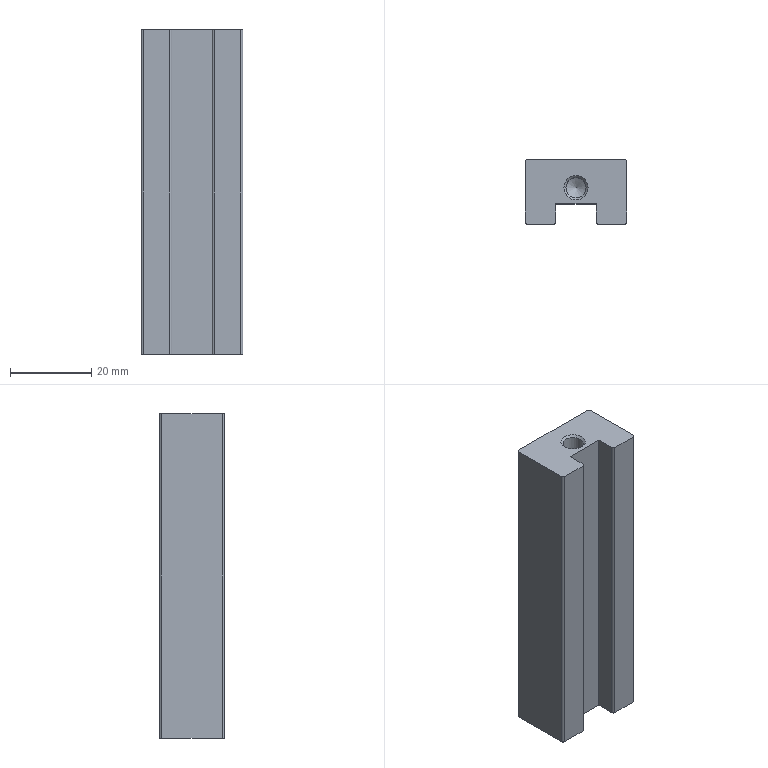Part | STEP file | 200 mesh_id1982 | 1 solid | 19 faces | box 25 x 16 x 80 mm | volume 27373 mm3 | plane 10 | cylinder 7 | cone 2 | commonest cylinder face diameters 1 x6 5 x1
STEP:
#1=CARTESIAN_POINT('',(-17200.384,-3959.169,0.));
#2=VERTEX_POINT('',#1);
#3=CARTESIAN_POINT('',(-17200.384,-3974.169,0.));
#4=VERTEX_POINT('',#3);
#5=CARTESIAN_POINT('',(-17200.384,-3959.169,0.));
#6=DIRECTION('',(0.,-1.,0.));
#7=VECTOR('',#6,1.);
#8=LINE('',#5,#7);
#9=EDGE_CURVE('',#2,#4,#8,.T.);
#10=ORIENTED_EDGE('',*,*,#9,.F.);
#11=CARTESIAN_POINT('',(-17200.384,-3959.169,80.));
#12=VERTEX_POINT('',#11);
#13=CARTESIAN_POINT('',(-17200.384,-3959.169,80.));
#14=DIRECTION('',(0.,0.,-1.));
#15=VECTOR('',#14,1.);
#16=LINE('',#13,#15);
#17=EDGE_CURVE('',#12,#2,#16,.T.);
#18=ORIENTED_EDGE('',*,*,#17,.F.);
#19=CARTESIAN_POINT('',(-17200.384,-3974.169,80.));
#20=VERTEX_POINT('',#19);
#21=CARTESIAN_POINT('',(-17200.384,-3959.169,80.));
#22=DIRECTION('',(0.,-1.,0.));
#23=VECTOR('',#22,1.);
#24=LINE('',#21,#23);
#25=EDGE_CURVE('',#12,#20,#24,.T.);
#26=ORIENTED_EDGE('',*,*,#25,.T.);
#27=CARTESIAN_POINT('',(-17200.384,-3974.169,80.));
#28=DIRECTION('',(0.,0.,-1.));
#29=VECTOR('',#28,1.);
#30=LINE('',#27,#29);
#31=EDGE_CURVE('',#20,#4,#30,.T.);
#32=ORIENTED_EDGE('',*,*,#31,.T.);
#33=EDGE_LOOP('',(#10,#18,#26,#32));
#34=FACE_OUTER_BOUND('',#33,.T.);
#35=CARTESIAN_POINT('',(-17200.384,-3959.169,80.));
#36=DIRECTION('',(1.,0.,0.));
#37=DIRECTION('',(0.,0.,1.));
#38=AXIS2_PLACEMENT_3D('',#35,#36,#37);
#39=PLANE('',#38);
#40=ADVANCED_FACE('',(#34),#39,.T.);
#41=CARTESIAN_POINT('',(-17200.884,-3974.669,0.));
#42=VERTEX_POINT('',#41);
#43=CARTESIAN_POINT('',(-17200.884,-3974.169,0.));
#44=DIRECTION('',(0.,0.,-1.));
#45=DIRECTION('',(1.,0.,0.));
#46=AXIS2_PLACEMENT_3D('',#43,#44,#45);
#47=CIRCLE('',#46,0.5);
#48=EDGE_CURVE('',#4,#42,#47,.T.);
#49=ORIENTED_EDGE('',*,*,#48,.F.);
#50=ORIENTED_EDGE('',*,*,#31,.F.);
#51=CARTESIAN_POINT('',(-17200.884,-3974.669,80.));
#52=VERTEX_POINT('',#51);
#53=CARTESIAN_POINT('',(-17200.884,-3974.169,80.));
#54=DIRECTION('',(0.,0.,-1.));
#55=DIRECTION('',(1.,0.,0.));
#56=AXIS2_PLACEMENT_3D('',#53,#54,#55);
#57=CIRCLE('',#56,0.5);
#58=EDGE_CURVE('',#20,#52,#57,.T.);
#59=ORIENTED_EDGE('',*,*,#58,.T.);
#60=CARTESIAN_POINT('',(-17200.884,-3974.669,80.));
#61=DIRECTION('',(0.,0.,-1.));
#62=VECTOR('',#61,1.);
#63=LINE('',#60,#62);
#64=EDGE_CURVE('',#52,#42,#63,.T.);
#65=ORIENTED_EDGE('',*,*,#64,.T.);
#66=EDGE_LOOP('',(#49,#50,#59,#65));
#67=FACE_OUTER_BOUND('',#66,.T.);
#68=CARTESIAN_POINT('',(-17200.884,-3974.169,80.));
#69=DIRECTION('',(0.,0.,-1.));
#70=DIRECTION('',(1.,0.,0.));
#71=AXIS2_PLACEMENT_3D('',#68,#69,#70);
#72=CYLINDRICAL_SURFACE('',#71,0.5);
#73=ADVANCED_FACE('',(#67),#72,.T.);
#74=CARTESIAN_POINT('',(-17207.384,-3974.669,0.));
#75=VERTEX_POINT('',#74);
#76=CARTESIAN_POINT('',(-17200.884,-3974.669,0.));
#77=DIRECTION('',(-1.,0.,0.));
#78=VECTOR('',#77,1.);
#79=LINE('',#76,#78);
#80=EDGE_CURVE('',#42,#75,#79,.T.);
#81=ORIENTED_EDGE('',*,*,#80,.F.);
#82=ORIENTED_EDGE('',*,*,#64,.F.);
#83=CARTESIAN_POINT('',(-17207.384,-3974.669,80.));
#84=VERTEX_POINT('',#83);
#85=CARTESIAN_POINT('',(-17200.884,-3974.669,80.));
#86=DIRECTION('',(-1.,0.,0.));
#87=VECTOR('',#86,1.);
#88=LINE('',#85,#87);
#89=EDGE_CURVE('',#52,#84,#88,.T.);
#90=ORIENTED_EDGE('',*,*,#89,.T.);
#91=CARTESIAN_POINT('',(-17207.384,-3974.669,80.));
#92=DIRECTION('',(0.,0.,-1.));
#93=VECTOR('',#92,1.);
#94=LINE('',#91,#93);
#95=EDGE_CURVE('',#84,#75,#94,.T.);
#96=ORIENTED_EDGE('',*,*,#95,.T.);
#97=EDGE_LOOP('',(#81,#82,#90,#96));
#98=FACE_OUTER_BOUND('',#97,.T.);
#99=CARTESIAN_POINT('',(-17200.884,-3974.669,80.));
#100=DIRECTION('',(0.,-1.,0.));
#101=DIRECTION('',(0.,0.,1.));
#102=AXIS2_PLACEMENT_3D('',#99,#100,#101);
#103=PLANE('',#102);
#104=ADVANCED_FACE('',(#98),#103,.T.);
#105=CARTESIAN_POINT('',(-17207.884,-3974.169,0.));
#106=VERTEX_POINT('',#105);
#107=CARTESIAN_POINT('',(-17207.384,-3974.169,0.));
#108=DIRECTION('',(0.,0.,-1.));
#109=DIRECTION('',(1.,0.,0.));
#110=AXIS2_PLACEMENT_3D('',#107,#108,#109);
#111=CIRCLE('',#110,0.5);
#112=EDGE_CURVE('',#75,#106,#111,.T.);
#113=ORIENTED_EDGE('',*,*,#112,.F.);
#114=ORIENTED_EDGE('',*,*,#95,.F.);
#115=CARTESIAN_POINT('',(-17207.884,-3974.169,80.));
#116=VERTEX_POINT('',#115);
#117=CARTESIAN_POINT('',(-17207.384,-3974.169,80.));
#118=DIRECTION('',(0.,0.,-1.));
#119=DIRECTION('',(1.,0.,0.));
#120=AXIS2_PLACEMENT_3D('',#117,#118,#119);
#121=CIRCLE('',#120,0.5);
#122=EDGE_CURVE('',#84,#116,#121,.T.);
#123=ORIENTED_EDGE('',*,*,#122,.T.);
#124=CARTESIAN_POINT('',(-17207.884,-3974.169,80.));
#125=DIRECTION('',(0.,0.,-1.));
#126=VECTOR('',#125,1.);
#127=LINE('',#124,#126);
#128=EDGE_CURVE('',#116,#106,#127,.T.);
#129=ORIENTED_EDGE('',*,*,#128,.T.);
#130=EDGE_LOOP('',(#113,#114,#123,#129));
#131=FACE_OUTER_BOUND('',#130,.T.);
#132=CARTESIAN_POINT('',(-17207.384,-3974.169,80.));
#133=DIRECTION('',(0.,0.,-1.));
#134=DIRECTION('',(1.,0.,0.));
#135=AXIS2_PLACEMENT_3D('',#132,#133,#134);
#136=CYLINDRICAL_SURFACE('',#135,0.5);
#137=ADVANCED_FACE('',(#131),#136,.T.);
#138=CARTESIAN_POINT('',(-17207.884,-3969.669,0.));
#139=VERTEX_POINT('',#138);
#140=CARTESIAN_POINT('',(-17207.884,-3974.169,0.));
#141=DIRECTION('',(0.,1.,0.));
#142=VECTOR('',#141,1.);
#143=LINE('',#140,#142);
#144=EDGE_CURVE('',#106,#139,#143,.T.);
#145=ORIENTED_EDGE('',*,*,#144,.F.);
#146=ORIENTED_EDGE('',*,*,#128,.F.);
#147=CARTESIAN_POINT('',(-17207.884,-3969.669,80.));
#148=VERTEX_POINT('',#147);
#149=CARTESIAN_POINT('',(-17207.884,-3974.169,80.));
#150=DIRECTION('',(0.,1.,0.));
#151=VECTOR('',#150,1.);
#152=LINE('',#149,#151);
#153=EDGE_CURVE('',#116,#148,#152,.T.);
#154=ORIENTED_EDGE('',*,*,#153,.T.);
#155=CARTESIAN_POINT('',(-17207.884,-3969.669,80.));
#156=DIRECTION('',(0.,0.,-1.));
#157=VECTOR('',#156,1.);
#158=LINE('',#155,#157);
#159=EDGE_CURVE('',#148,#139,#158,.T.);
#160=ORIENTED_EDGE('',*,*,#159,.T.);
#161=EDGE_LOOP('',(#145,#146,#154,#160));
#162=FACE_OUTER_BOUND('',#161,.T.);
#163=CARTESIAN_POINT('',(-17207.884,-3974.169,80.));
#164=DIRECTION('',(-1.,0.,0.));
#165=DIRECTION('',(0.,0.,-1.));
#166=AXIS2_PLACEMENT_3D('',#163,#164,#165);
#167=PLANE('',#166);
#168=ADVANCED_FACE('',(#162),#167,.T.);
#169=CARTESIAN_POINT('',(-17217.884,-3969.669,0.));
#170=VERTEX_POINT('',#169);
#171=CARTESIAN_POINT('',(-17207.884,-3969.669,0.));
#172=DIRECTION('',(-1.,0.,0.));
#173=VECTOR('',#172,1.);
#174=LINE('',#171,#173);
#175=EDGE_CURVE('',#139,#170,#174,.T.);
#176=ORIENTED_EDGE('',*,*,#175,.F.);
#177=ORIENTED_EDGE('',*,*,#159,.F.);
#178=CARTESIAN_POINT('',(-17217.884,-3969.669,80.));
#179=VERTEX_POINT('',#178);
#180=CARTESIAN_POINT('',(-17207.884,-3969.669,80.));
#181=DIRECTION('',(-1.,0.,0.));
#182=VECTOR('',#181,1.);
#183=LINE('',#180,#182);
#184=EDGE_CURVE('',#148,#179,#183,.T.);
#185=ORIENTED_EDGE('',*,*,#184,.T.);
#186=CARTESIAN_POINT('',(-17217.884,-3969.669,80.));
#187=DIRECTION('',(0.,0.,-1.));
#188=VECTOR('',#187,1.);
#189=LINE('',#186,#188);
#190=EDGE_CURVE('',#179,#170,#189,.T.);
#191=ORIENTED_EDGE('',*,*,#190,.T.);
#192=EDGE_LOOP('',(#176,#177,#185,#191));
#193=FACE_OUTER_BOUND('',#192,.T.);
#194=CARTESIAN_POINT('',(-17207.884,-3969.669,80.));
#195=DIRECTION('',(0.,-1.,0.));
#196=DIRECTION('',(0.,0.,1.));
#197=AXIS2_PLACEMENT_3D('',#194,#195,#196);
#198=PLANE('',#197);
#199=ADVANCED_FACE('',(#193),#198,.T.);
#200=CARTESIAN_POINT('',(-17217.884,-3974.169,0.));
#201=VERTEX_POINT('',#200);
#202=CARTESIAN_POINT('',(-17217.884,-3969.669,0.));
#203=DIRECTION('',(0.,-1.,0.));
#204=VECTOR('',#203,1.);
#205=LINE('',#202,#204);
#206=EDGE_CURVE('',#170,#201,#205,.T.);
#207=ORIENTED_EDGE('',*,*,#206,.F.);
#208=ORIENTED_EDGE('',*,*,#190,.F.);
#209=CARTESIAN_POINT('',(-17217.884,-3974.169,80.));
#210=VERTEX_POINT('',#209);
#211=CARTESIAN_POINT('',(-17217.884,-3969.669,80.));
#212=DIRECTION('',(0.,-1.,0.));
#213=VECTOR('',#212,1.);
#214=LINE('',#211,#213);
#215=EDGE_CURVE('',#179,#210,#214,.T.);
#216=ORIENTED_EDGE('',*,*,#215,.T.);
#217=CARTESIAN_POINT('',(-17217.884,-3974.169,80.));
#218=DIRECTION('',(0.,0.,-1.));
#219=VECTOR('',#218,1.);
#220=LINE('',#217,#219);
#221=EDGE_CURVE('',#210,#201,#220,.T.);
#222=ORIENTED_EDGE('',*,*,#221,.T.);
#223=EDGE_LOOP('',(#207,#208,#216,#222));
#224=FACE_OUTER_BOUND('',#223,.T.);
#225=CARTESIAN_POINT('',(-17217.884,-3969.669,80.));
#226=DIRECTION('',(1.,0.,0.));
#227=DIRECTION('',(0.,0.,1.));
#228=AXIS2_PLACEMENT_3D('',#225,#226,#227);
#229=PLANE('',#228);
#230=ADVANCED_FACE('',(#224),#229,.T.);
#231=CARTESIAN_POINT('',(-17218.384,-3974.669,0.));
#232=VERTEX_POINT('',#231);
#233=CARTESIAN_POINT('',(-17218.384,-3974.169,0.));
#234=DIRECTION('',(0.,0.,-1.));
#235=DIRECTION('',(1.,0.,0.));
#236=AXIS2_PLACEMENT_3D('',#233,#234,#235);
#237=CIRCLE('',#236,0.5);
#238=EDGE_CURVE('',#201,#232,#237,.T.);
#239=ORIENTED_EDGE('',*,*,#238,.F.);
#240=ORIENTED_EDGE('',*,*,#221,.F.);
#241=CARTESIAN_POINT('',(-17218.384,-3974.669,80.));
#242=VERTEX_POINT('',#241);
#243=CARTESIAN_POINT('',(-17218.384,-3974.169,80.));
#244=DIRECTION('',(0.,0.,-1.));
#245=DIRECTION('',(1.,0.,0.));
#246=AXIS2_PLACEMENT_3D('',#243,#244,#245);
#247=CIRCLE('',#246,0.5);
#248=EDGE_CURVE('',#210,#242,#247,.T.);
#249=ORIENTED_EDGE('',*,*,#248,.T.);
#250=CARTESIAN_POINT('',(-17218.384,-3974.669,80.));
#251=DIRECTION('',(0.,0.,-1.));
#252=VECTOR('',#251,1.);
#253=LINE('',#250,#252);
#254=EDGE_CURVE('',#242,#232,#253,.T.);
#255=ORIENTED_EDGE('',*,*,#254,.T.);
#256=EDGE_LOOP('',(#239,#240,#249,#255));
#257=FACE_OUTER_BOUND('',#256,.T.);
#258=CARTESIAN_POINT('',(-17218.384,-3974.169,80.));
#259=DIRECTION('',(0.,0.,-1.));
#260=DIRECTION('',(1.,0.,0.));
#261=AXIS2_PLACEMENT_3D('',#258,#259,#260);
#262=CYLINDRICAL_SURFACE('',#261,0.5);
#263=ADVANCED_FACE('',(#257),#262,.T.);
#264=CARTESIAN_POINT('',(-17224.884,-3974.669,0.));
#265=VERTEX_POINT('',#264);
#266=CARTESIAN_POINT('',(-17218.384,-3974.669,0.));
#267=DIRECTION('',(-1.,0.,0.));
#268=VECTOR('',#267,1.);
#269=LINE('',#266,#268);
#270=EDGE_CURVE('',#232,#265,#269,.T.);
#271=ORIENTED_EDGE('',*,*,#270,.F.);
#272=ORIENTED_EDGE('',*,*,#254,.F.);
#273=CARTESIAN_POINT('',(-17224.884,-3974.669,80.));
#274=VERTEX_POINT('',#273);
#275=CARTESIAN_POINT('',(-17218.384,-3974.669,80.));
#276=DIRECTION('',(-1.,0.,0.));
#277=VECTOR('',#276,1.);
#278=LINE('',#275,#277);
#279=EDGE_CURVE('',#242,#274,#278,.T.);
#280=ORIENTED_EDGE('',*,*,#279,.T.);
#281=CARTESIAN_POINT('',(-17224.884,-3974.669,80.));
#282=DIRECTION('',(0.,0.,-1.));
#283=VECTOR('',#282,1.);
#284=LINE('',#281,#283);
#285=EDGE_CURVE('',#274,#265,#284,.T.);
#286=ORIENTED_EDGE('',*,*,#285,.T.);
#287=EDGE_LOOP('',(#271,#272,#280,#286));
#288=FACE_OUTER_BOUND('',#287,.T.);
#289=CARTESIAN_POINT('',(-17218.384,-3974.669,80.));
#290=DIRECTION('',(0.,-1.,0.));
#291=DIRECTION('',(0.,0.,1.));
#292=AXIS2_PLACEMENT_3D('',#289,#290,#291);
#293=PLANE('',#292);
#294=ADVANCED_FACE('',(#288),#293,.T.);
#295=CARTESIAN_POINT('',(-17225.384,-3974.169,0.));
#296=VERTEX_POINT('',#295);
#297=CARTESIAN_POINT('',(-17224.884,-3974.169,0.));
#298=DIRECTION('',(0.,0.,-1.));
#299=DIRECTION('',(1.,0.,0.));
#300=AXIS2_PLACEMENT_3D('',#297,#298,#299);
#301=CIRCLE('',#300,0.5);
#302=EDGE_CURVE('',#265,#296,#301,.T.);
#303=ORIENTED_EDGE('',*,*,#302,.F.);
#304=ORIENTED_EDGE('',*,*,#285,.F.);
#305=CARTESIAN_POINT('',(-17225.384,-3974.169,80.));
#306=VERTEX_POINT('',#305);
#307=CARTESIAN_POINT('',(-17224.884,-3974.169,80.));
#308=DIRECTION('',(0.,0.,-1.));
#309=DIRECTION('',(1.,0.,0.));
#310=AXIS2_PLACEMENT_3D('',#307,#308,#309);
#311=CIRCLE('',#310,0.5);
#312=EDGE_CURVE('',#274,#306,#311,.T.);
#313=ORIENTED_EDGE('',*,*,#312,.T.);
#314=CARTESIAN_POINT('',(-17225.384,-3974.169,80.));
#315=DIRECTION('',(0.,0.,-1.));
#316=VECTOR('',#315,1.);
#317=LINE('',#314,#316);
#318=EDGE_CURVE('',#306,#296,#317,.T.);
#319=ORIENTED_EDGE('',*,*,#318,.T.);
#320=EDGE_LOOP('',(#303,#304,#313,#319));
#321=FACE_OUTER_BOUND('',#320,.T.);
#322=CARTESIAN_POINT('',(-17224.884,-3974.169,80.));
#323=DIRECTION('',(0.,0.,-1.));
#324=DIRECTION('',(1.,0.,0.));
#325=AXIS2_PLACEMENT_3D('',#322,#323,#324);
#326=CYLINDRICAL_SURFACE('',#325,0.5);
#327=ADVANCED_FACE('',(#321),#326,.T.);
#328=CARTESIAN_POINT('',(-17225.384,-3959.169,0.));
#329=VERTEX_POINT('',#328);
#330=CARTESIAN_POINT('',(-17225.384,-3974.169,0.));
#331=DIRECTION('',(0.,1.,0.));
#332=VECTOR('',#331,1.);
#333=LINE('',#330,#332);
#334=EDGE_CURVE('',#296,#329,#333,.T.);
#335=ORIENTED_EDGE('',*,*,#334,.F.);
#336=ORIENTED_EDGE('',*,*,#318,.F.);
#337=CARTESIAN_POINT('',(-17225.384,-3959.169,80.));
#338=VERTEX_POINT('',#337);
#339=CARTESIAN_POINT('',(-17225.384,-3974.169,80.));
#340=DIRECTION('',(0.,1.,0.));
#341=VECTOR('',#340,1.);
#342=LINE('',#339,#341);
#343=EDGE_CURVE('',#306,#338,#342,.T.);
#344=ORIENTED_EDGE('',*,*,#343,.T.);
#345=CARTESIAN_POINT('',(-17225.384,-3959.169,80.));
#346=DIRECTION('',(0.,0.,-1.));
#347=VECTOR('',#346,1.);
#348=LINE('',#345,#347);
#349=EDGE_CURVE('',#338,#329,#348,.T.);
#350=ORIENTED_EDGE('',*,*,#349,.T.);
#351=EDGE_LOOP('',(#335,#336,#344,#350));
#352=FACE_OUTER_BOUND('',#351,.T.);
#353=CARTESIAN_POINT('',(-17225.384,-3974.169,80.));
#354=DIRECTION('',(-1.,0.,0.));
#355=DIRECTION('',(0.,0.,-1.));
#356=AXIS2_PLACEMENT_3D('',#353,#354,#355);
#357=PLANE('',#356);
#358=ADVANCED_FACE('',(#352),#357,.T.);
#359=CARTESIAN_POINT('',(-17224.884,-3958.669,0.));
#360=VERTEX_POINT('',#359);
#361=CARTESIAN_POINT('',(-17224.884,-3959.169,0.));
#362=DIRECTION('',(0.,0.,-1.));
#363=DIRECTION('',(1.,0.,0.));
#364=AXIS2_PLACEMENT_3D('',#361,#362,#363);
#365=CIRCLE('',#364,0.5);
#366=EDGE_CURVE('',#329,#360,#365,.T.);
#367=ORIENTED_EDGE('',*,*,#366,.F.);
#368=ORIENTED_EDGE('',*,*,#349,.F.);
#369=CARTESIAN_POINT('',(-17224.884,-3958.669,80.));
#370=VERTEX_POINT('',#369);
#371=CARTESIAN_POINT('',(-17224.884,-3959.169,80.));
#372=DIRECTION('',(0.,0.,-1.));
#373=DIRECTION('',(1.,0.,0.));
#374=AXIS2_PLACEMENT_3D('',#371,#372,#373);
#375=CIRCLE('',#374,0.5);
#376=EDGE_CURVE('',#338,#370,#375,.T.);
#377=ORIENTED_EDGE('',*,*,#376,.T.);
#378=CARTESIAN_POINT('',(-17224.884,-3958.669,80.));
#379=DIRECTION('',(0.,0.,-1.));
#380=VECTOR('',#379,1.);
#381=LINE('',#378,#380);
#382=EDGE_CURVE('',#370,#360,#381,.T.);
#383=ORIENTED_EDGE('',*,*,#382,.T.);
#384=EDGE_LOOP('',(#367,#368,#377,#383));
#385=FACE_OUTER_BOUND('',#384,.T.);
#386=CARTESIAN_POINT('',(-17224.884,-3959.169,80.));
#387=DIRECTION('',(0.,0.,-1.));
#388=DIRECTION('',(1.,0.,0.));
#389=AXIS2_PLACEMENT_3D('',#386,#387,#388);
#390=CYLINDRICAL_SURFACE('',#389,0.5);
#391=ADVANCED_FACE('',(#385),#390,.T.);
#392=CARTESIAN_POINT('',(-17200.884,-3958.669,0.));
#393=VERTEX_POINT('',#392);
#394=CARTESIAN_POINT('',(-17224.884,-3958.669,0.));
#395=DIRECTION('',(1.,0.,0.));
#396=VECTOR('',#395,1.);
#397=LINE('',#394,#396);
#398=EDGE_CURVE('',#360,#393,#397,.T.);
#399=ORIENTED_EDGE('',*,*,#398,.F.);
#400=ORIENTED_EDGE('',*,*,#382,.F.);
#401=CARTESIAN_POINT('',(-17200.884,-3958.669,80.));
#402=VERTEX_POINT('',#401);
#403=CARTESIAN_POINT('',(-17224.884,-3958.669,80.));
#404=DIRECTION('',(1.,0.,0.));
#405=VECTOR('',#404,1.);
#406=LINE('',#403,#405);
#407=EDGE_CURVE('',#370,#402,#406,.T.);
#408=ORIENTED_EDGE('',*,*,#407,.T.);
#409=CARTESIAN_POINT('',(-17200.884,-3958.669,80.));
#410=DIRECTION('',(0.,0.,-1.));
#411=VECTOR('',#410,1.);
#412=LINE('',#409,#411);
#413=EDGE_CURVE('',#402,#393,#412,.T.);
#414=ORIENTED_EDGE('',*,*,#413,.T.);
#415=EDGE_LOOP('',(#399,#400,#408,#414));
#416=FACE_OUTER_BOUND('',#415,.T.);
#417=CARTESIAN_POINT('',(-17224.884,-3958.669,80.));
#418=DIRECTION('',(0.,1.,0.));
#419=DIRECTION('',(0.,0.,-1.));
#420=AXIS2_PLACEMENT_3D('',#417,#418,#419);
#421=PLANE('',#420);
#422=ADVANCED_FACE('',(#416),#421,.T.);
#423=CARTESIAN_POINT('',(-17200.884,-3959.169,0.));
#424=DIRECTION('',(0.,0.,-1.));
#425=DIRECTION('',(1.,0.,0.));
#426=AXIS2_PLACEMENT_3D('',#423,#424,#425);
#427=CIRCLE('',#426,0.5);
#428=EDGE_CURVE('',#393,#2,#427,.T.);
#429=ORIENTED_EDGE('',*,*,#428,.F.);
#430=ORIENTED_EDGE('',*,*,#413,.F.);
#431=CARTESIAN_POINT('',(-17200.884,-3959.169,80.));
#432=DIRECTION('',(0.,0.,-1.));
#433=DIRECTION('',(1.,0.,0.));
#434=AXIS2_PLACEMENT_3D('',#431,#432,#433);
#435=CIRCLE('',#434,0.5);
#436=EDGE_CURVE('',#402,#12,#435,.T.);
#437=ORIENTED_EDGE('',*,*,#436,.T.);
#438=ORIENTED_EDGE('',*,*,#17,.T.);
#439=EDGE_LOOP('',(#429,#430,#437,#438));
#440=FACE_OUTER_BOUND('',#439,.T.);
#441=CARTESIAN_POINT('',(-17200.884,-3959.169,80.));
#442=DIRECTION('',(0.,0.,-1.));
#443=DIRECTION('',(1.,0.,0.));
#444=AXIS2_PLACEMENT_3D('',#441,#442,#443);
#445=CYLINDRICAL_SURFACE('',#444,0.5);
#446=ADVANCED_FACE('',(#440),#445,.T.);
#447=CARTESIAN_POINT('',(-17215.884,-3965.669,80.));
#448=VERTEX_POINT('',#447);
#449=CARTESIAN_POINT('',(-17212.884,-3965.669,80.));
#450=DIRECTION('',(0.,0.,-1.));
#451=DIRECTION('',(-1.,0.,0.));
#452=AXIS2_PLACEMENT_3D('',#449,#450,#451);
#453=CIRCLE('',#452,3.);
#454=EDGE_CURVE('',#448,#448,#453,.T.);
#455=ORIENTED_EDGE('',*,*,#454,.T.);
#456=EDGE_LOOP('',(#455));
#457=FACE_BOUND('',#456,.T.);
#458=ORIENTED_EDGE('',*,*,#25,.F.);
#459=ORIENTED_EDGE('',*,*,#436,.F.);
#460=ORIENTED_EDGE('',*,*,#407,.F.);
#461=ORIENTED_EDGE('',*,*,#376,.F.);
#462=ORIENTED_EDGE('',*,*,#343,.F.);
#463=ORIENTED_EDGE('',*,*,#312,.F.);
#464=ORIENTED_EDGE('',*,*,#279,.F.);
#465=ORIENTED_EDGE('',*,*,#248,.F.);
#466=ORIENTED_EDGE('',*,*,#215,.F.);
#467=ORIENTED_EDGE('',*,*,#184,.F.);
#468=ORIENTED_EDGE('',*,*,#153,.F.);
#469=ORIENTED_EDGE('',*,*,#122,.F.);
#470=ORIENTED_EDGE('',*,*,#89,.F.);
#471=ORIENTED_EDGE('',*,*,#58,.F.);
#472=EDGE_LOOP('',(#458,#459,#460,#461,#462,#463,#464,#465,#466,#467,#468,#469,#470,#471));
#473=FACE_BOUND('',#472,.T.);
#474=CARTESIAN_POINT('',(-17200.884,-3974.169,80.));
#475=DIRECTION('',(0.,0.,-1.));
#476=DIRECTION('',(1.,0.,0.));
#477=AXIS2_PLACEMENT_3D('',#474,#475,#476);
#478=PLANE('',#477);
#479=ADVANCED_FACE('',(#457,#473),#478,.F.);
#480=ORIENTED_EDGE('',*,*,#9,.T.);
#481=ORIENTED_EDGE('',*,*,#48,.T.);
#482=ORIENTED_EDGE('',*,*,#80,.T.);
#483=ORIENTED_EDGE('',*,*,#112,.T.);
#484=ORIENTED_EDGE('',*,*,#144,.T.);
#485=ORIENTED_EDGE('',*,*,#175,.T.);
#486=ORIENTED_EDGE('',*,*,#206,.T.);
#487=ORIENTED_EDGE('',*,*,#238,.T.);
#488=ORIENTED_EDGE('',*,*,#270,.T.);
#489=ORIENTED_EDGE('',*,*,#302,.T.);
#490=ORIENTED_EDGE('',*,*,#334,.T.);
#491=ORIENTED_EDGE('',*,*,#366,.T.);
#492=ORIENTED_EDGE('',*,*,#398,.T.);
#493=ORIENTED_EDGE('',*,*,#428,.T.);
#494=EDGE_LOOP('',(#480,#481,#482,#483,#484,#485,#486,#487,#488,#489,#490,#491,#492,#493));
#495=FACE_OUTER_BOUND('',#494,.T.);
#496=CARTESIAN_POINT('',(-17200.884,-3974.169,0.));
#497=DIRECTION('',(0.,0.,-1.));
#498=DIRECTION('',(1.,0.,0.));
#499=AXIS2_PLACEMENT_3D('',#496,#497,#498);
#500=PLANE('',#499);
#501=ADVANCED_FACE('',(#495),#500,.T.);
#502=CARTESIAN_POINT('',(-17215.384,-3965.669,50.));
#503=VERTEX_POINT('',#502);
#504=CARTESIAN_POINT('',(-17212.884,-3965.669,50.));
#505=DIRECTION('',(0.,0.,1.));
#506=DIRECTION('',(-1.,0.,0.));
#507=AXIS2_PLACEMENT_3D('',#504,#505,#506);
#508=CIRCLE('',#507,2.5);
#509=EDGE_CURVE('',#503,#503,#508,.T.);
#510=ORIENTED_EDGE('',*,*,#509,.T.);
#511=EDGE_LOOP('',(#510));
#512=FACE_BOUND('',#511,.T.);
#513=CARTESIAN_POINT('',(-17212.884,-3965.669,48.498));
#514=VERTEX_POINT('',#513);
#515=VERTEX_LOOP('',#514);
#516=FACE_BOUND('',#515,.T.);
#517=CARTESIAN_POINT('',(-17212.884,-3965.669,50.));
#518=DIRECTION('',(0.,0.,1.));
#519=DIRECTION('',(-1.,0.,0.));
#520=AXIS2_PLACEMENT_3D('',#517,#518,#519);
#521=CONICAL_SURFACE('',#520,2.5,59.);
#522=ADVANCED_FACE('',(#512,#516),#521,.F.);
#523=CARTESIAN_POINT('',(-17215.384,-3965.669,79.5));
#524=VERTEX_POINT('',#523);
#525=CARTESIAN_POINT('',(-17212.884,-3965.669,79.5));
#526=DIRECTION('',(0.,0.,1.));
#527=DIRECTION('',(-1.,0.,0.));
#528=AXIS2_PLACEMENT_3D('',#525,#526,#527);
#529=CIRCLE('',#528,2.5);
#530=EDGE_CURVE('',#524,#524,#529,.T.);
#531=ORIENTED_EDGE('',*,*,#530,.T.);
#532=EDGE_LOOP('',(#531));
#533=FACE_BOUND('',#532,.T.);
#534=ORIENTED_EDGE('',*,*,#509,.F.);
#535=EDGE_LOOP('',(#534));
#536=FACE_BOUND('',#535,.T.);
#537=CARTESIAN_POINT('',(-17212.884,-3965.669,80.));
#538=DIRECTION('',(0.,0.,-1.));
#539=DIRECTION('',(1.,0.,0.));
#540=AXIS2_PLACEMENT_3D('',#537,#538,#539);
#541=CYLINDRICAL_SURFACE('',#540,2.5);
#542=ADVANCED_FACE('',(#533,#536),#541,.F.);
#543=ORIENTED_EDGE('',*,*,#530,.F.);
#544=EDGE_LOOP('',(#543));
#545=FACE_BOUND('',#544,.T.);
#546=ORIENTED_EDGE('',*,*,#454,.F.);
#547=EDGE_LOOP('',(#546));
#548=FACE_BOUND('',#547,.T.);
#549=CARTESIAN_POINT('',(-17212.884,-3965.669,80.));
#550=DIRECTION('',(0.,0.,1.));
#551=DIRECTION('',(-1.,0.,0.));
#552=AXIS2_PLACEMENT_3D('',#549,#550,#551);
#553=CONICAL_SURFACE('',#552,3.,45.);
#554=ADVANCED_FACE('',(#545,#548),#553,.F.);
#555=CLOSED_SHELL('',(#40,#73,#104,#137,#168,#199,#230,#263,#294,#327,#358,#391,#422,#446,#479,#501,#522,#542,#554));
#556=MANIFOLD_SOLID_BREP('',#555);
#557=(LENGTH_UNIT()NAMED_UNIT(*)SI_UNIT(.MILLI.,.METRE.));
#558=UNCERTAINTY_MEASURE_WITH_UNIT(LENGTH_MEASURE(0.00002),#557,'','');
#559=(NAMED_UNIT(*)PLANE_ANGLE_UNIT()SI_UNIT($,.RADIAN.));
#560=PLANE_ANGLE_MEASURE_WITH_UNIT(PLANE_ANGLE_MEASURE(0.01745),#559);
#561=DIMENSIONAL_EXPONENTS(0.,0.,0.,0.,0.,0.,0.);
#562=(CONVERSION_BASED_UNIT('DEGREE',#560)NAMED_UNIT(#561)PLANE_ANGLE_UNIT());
#563=(NAMED_UNIT(*)SI_UNIT($,.STERADIAN.)SOLID_ANGLE_UNIT());
#564=(GEOMETRIC_REPRESENTATION_CONTEXT(3)GLOBAL_UNCERTAINTY_ASSIGNED_CONTEXT((#558))GLOBAL_UNIT_ASSIGNED_CONTEXT((#557,#562,#563))REPRESENTATION_CONTEXT('',''));
#565=ADVANCED_BREP_SHAPE_REPRESENTATION('',(#556),#564);